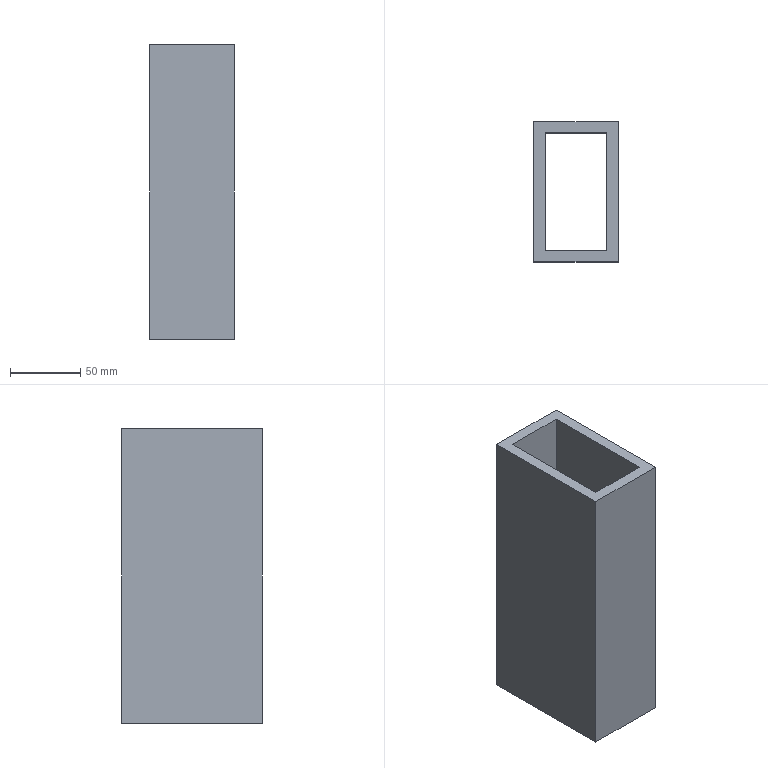Part | SolidWorks | features BaseBody 1 | 1 solid | 10 faces | box 60 x 100 x 210 mm | volume 483840 mm3 | plane 10
STEP:
#1=CARTESIAN_POINT('',(-30.,50.,-105.));
#2=VERTEX_POINT('',#1);
#3=CARTESIAN_POINT('',(-30.,50.,105.));
#4=VERTEX_POINT('',#3);
#5=CARTESIAN_POINT('',(-30.,50.,-105.));
#6=DIRECTION('',(0.,0.,1.));
#7=VECTOR('',#6,1000.);
#8=LINE('',#5,#7);
#9=EDGE_CURVE('',#2,#4,#8,.T.);
#10=ORIENTED_EDGE('',*,*,#9,.F.);
#11=CARTESIAN_POINT('',(-30.,-50.,-105.));
#12=VERTEX_POINT('',#11);
#13=CARTESIAN_POINT('',(-30.,-50.,-105.));
#14=DIRECTION('',(0.,1.,0.));
#15=VECTOR('',#14,1000.);
#16=LINE('',#13,#15);
#17=EDGE_CURVE('',#12,#2,#16,.T.);
#18=ORIENTED_EDGE('',*,*,#17,.F.);
#19=CARTESIAN_POINT('',(-30.,-50.,105.));
#20=VERTEX_POINT('',#19);
#21=CARTESIAN_POINT('',(-30.,-50.,-105.));
#22=DIRECTION('',(0.,0.,-1.));
#23=VECTOR('',#22,1000.);
#24=LINE('',#21,#23);
#25=EDGE_CURVE('',#20,#12,#24,.T.);
#26=ORIENTED_EDGE('',*,*,#25,.F.);
#27=CARTESIAN_POINT('',(-30.,-50.,105.));
#28=DIRECTION('',(0.,-1.,0.));
#29=VECTOR('',#28,1000.);
#30=LINE('',#27,#29);
#31=EDGE_CURVE('',#4,#20,#30,.T.);
#32=ORIENTED_EDGE('',*,*,#31,.F.);
#33=EDGE_LOOP('',(#10,#18,#26,#32));
#34=FACE_OUTER_BOUND('',#33,.T.);
#35=CARTESIAN_POINT('',(-30.,-50.,-105.));
#36=DIRECTION('',(1.,0.,0.));
#37=DIRECTION('',(0.,0.,-1.));
#38=AXIS2_PLACEMENT_3D('',#35,#36,#37);
#39=PLANE('',#38);
#40=ADVANCED_FACE('',(#34),#39,.F.);
#41=CARTESIAN_POINT('',(-22.,42.,105.));
#42=VERTEX_POINT('',#41);
#43=CARTESIAN_POINT('',(22.,42.,105.));
#44=VERTEX_POINT('',#43);
#45=CARTESIAN_POINT('',(-30.,42.,105.));
#46=DIRECTION('',(1.,0.,0.));
#47=VECTOR('',#46,1000.);
#48=LINE('',#45,#47);
#49=EDGE_CURVE('',#42,#44,#48,.T.);
#50=ORIENTED_EDGE('',*,*,#49,.T.);
#51=CARTESIAN_POINT('',(22.,-42.,105.));
#52=VERTEX_POINT('',#51);
#53=CARTESIAN_POINT('',(22.,-50.,105.));
#54=DIRECTION('',(0.,-1.,0.));
#55=VECTOR('',#54,1000.);
#56=LINE('',#53,#55);
#57=EDGE_CURVE('',#44,#52,#56,.T.);
#58=ORIENTED_EDGE('',*,*,#57,.T.);
#59=CARTESIAN_POINT('',(-22.,-42.,105.));
#60=VERTEX_POINT('',#59);
#61=CARTESIAN_POINT('',(-30.,-42.,105.));
#62=DIRECTION('',(-1.,0.,0.));
#63=VECTOR('',#62,1000.);
#64=LINE('',#61,#63);
#65=EDGE_CURVE('',#52,#60,#64,.T.);
#66=ORIENTED_EDGE('',*,*,#65,.T.);
#67=CARTESIAN_POINT('',(-22.,-50.,105.));
#68=DIRECTION('',(0.,1.,0.));
#69=VECTOR('',#68,1000.);
#70=LINE('',#67,#69);
#71=EDGE_CURVE('',#60,#42,#70,.T.);
#72=ORIENTED_EDGE('',*,*,#71,.T.);
#73=EDGE_LOOP('',(#50,#58,#66,#72));
#74=FACE_BOUND('',#73,.T.);
#75=CARTESIAN_POINT('',(30.,-50.,105.));
#76=VERTEX_POINT('',#75);
#77=CARTESIAN_POINT('',(30.,50.,105.));
#78=VERTEX_POINT('',#77);
#79=CARTESIAN_POINT('',(30.,-50.,105.));
#80=DIRECTION('',(0.,1.,0.));
#81=VECTOR('',#80,1000.);
#82=LINE('',#79,#81);
#83=EDGE_CURVE('',#76,#78,#82,.T.);
#84=ORIENTED_EDGE('',*,*,#83,.T.);
#85=CARTESIAN_POINT('',(-30.,50.,105.));
#86=DIRECTION('',(-1.,0.,0.));
#87=VECTOR('',#86,1000.);
#88=LINE('',#85,#87);
#89=EDGE_CURVE('',#78,#4,#88,.T.);
#90=ORIENTED_EDGE('',*,*,#89,.T.);
#91=ORIENTED_EDGE('',*,*,#31,.T.);
#92=CARTESIAN_POINT('',(-30.,-50.,105.));
#93=DIRECTION('',(1.,0.,0.));
#94=VECTOR('',#93,1000.);
#95=LINE('',#92,#94);
#96=EDGE_CURVE('',#20,#76,#95,.T.);
#97=ORIENTED_EDGE('',*,*,#96,.T.);
#98=EDGE_LOOP('',(#84,#90,#91,#97));
#99=FACE_OUTER_BOUND('',#98,.T.);
#100=CARTESIAN_POINT('',(-30.,-50.,105.));
#101=DIRECTION('',(0.,0.,1.));
#102=DIRECTION('',(1.,0.,0.));
#103=AXIS2_PLACEMENT_3D('',#100,#101,#102);
#104=PLANE('',#103);
#105=ADVANCED_FACE('',(#74,#99),#104,.T.);
#106=ORIENTED_EDGE('',*,*,#89,.F.);
#107=CARTESIAN_POINT('',(30.,50.,-105.));
#108=VERTEX_POINT('',#107);
#109=CARTESIAN_POINT('',(30.,50.,-105.));
#110=DIRECTION('',(0.,0.,-1.));
#111=VECTOR('',#110,1000.);
#112=LINE('',#109,#111);
#113=EDGE_CURVE('',#78,#108,#112,.T.);
#114=ORIENTED_EDGE('',*,*,#113,.T.);
#115=CARTESIAN_POINT('',(-30.,50.,-105.));
#116=DIRECTION('',(-1.,0.,0.));
#117=VECTOR('',#116,1000.);
#118=LINE('',#115,#117);
#119=EDGE_CURVE('',#108,#2,#118,.T.);
#120=ORIENTED_EDGE('',*,*,#119,.T.);
#121=ORIENTED_EDGE('',*,*,#9,.T.);
#122=EDGE_LOOP('',(#106,#114,#120,#121));
#123=FACE_OUTER_BOUND('',#122,.T.);
#124=CARTESIAN_POINT('',(-30.,50.,-105.));
#125=DIRECTION('',(0.,1.,0.));
#126=DIRECTION('',(0.,0.,1.));
#127=AXIS2_PLACEMENT_3D('',#124,#125,#126);
#128=PLANE('',#127);
#129=ADVANCED_FACE('',(#123),#128,.T.);
#130=CARTESIAN_POINT('',(-22.,42.,-105.));
#131=VERTEX_POINT('',#130);
#132=CARTESIAN_POINT('',(22.,42.,-105.));
#133=VERTEX_POINT('',#132);
#134=CARTESIAN_POINT('',(-30.,42.,-105.));
#135=DIRECTION('',(1.,0.,0.));
#136=VECTOR('',#135,1000.);
#137=LINE('',#134,#136);
#138=EDGE_CURVE('',#131,#133,#137,.T.);
#139=ORIENTED_EDGE('',*,*,#138,.F.);
#140=CARTESIAN_POINT('',(-22.,-42.,-105.));
#141=VERTEX_POINT('',#140);
#142=CARTESIAN_POINT('',(-22.,-50.,-105.));
#143=DIRECTION('',(0.,1.,0.));
#144=VECTOR('',#143,1000.);
#145=LINE('',#142,#144);
#146=EDGE_CURVE('',#141,#131,#145,.T.);
#147=ORIENTED_EDGE('',*,*,#146,.F.);
#148=CARTESIAN_POINT('',(22.,-42.,-105.));
#149=VERTEX_POINT('',#148);
#150=CARTESIAN_POINT('',(-30.,-42.,-105.));
#151=DIRECTION('',(-1.,0.,0.));
#152=VECTOR('',#151,1000.);
#153=LINE('',#150,#152);
#154=EDGE_CURVE('',#149,#141,#153,.T.);
#155=ORIENTED_EDGE('',*,*,#154,.F.);
#156=CARTESIAN_POINT('',(22.,-50.,-105.));
#157=DIRECTION('',(0.,-1.,0.));
#158=VECTOR('',#157,1000.);
#159=LINE('',#156,#158);
#160=EDGE_CURVE('',#133,#149,#159,.T.);
#161=ORIENTED_EDGE('',*,*,#160,.F.);
#162=EDGE_LOOP('',(#139,#147,#155,#161));
#163=FACE_BOUND('',#162,.T.);
#164=CARTESIAN_POINT('',(30.,-50.,-105.));
#165=VERTEX_POINT('',#164);
#166=CARTESIAN_POINT('',(30.,-50.,-105.));
#167=DIRECTION('',(0.,1.,0.));
#168=VECTOR('',#167,1000.);
#169=LINE('',#166,#168);
#170=EDGE_CURVE('',#165,#108,#169,.T.);
#171=ORIENTED_EDGE('',*,*,#170,.F.);
#172=CARTESIAN_POINT('',(-30.,-50.,-105.));
#173=DIRECTION('',(1.,0.,0.));
#174=VECTOR('',#173,1000.);
#175=LINE('',#172,#174);
#176=EDGE_CURVE('',#12,#165,#175,.T.);
#177=ORIENTED_EDGE('',*,*,#176,.F.);
#178=ORIENTED_EDGE('',*,*,#17,.T.);
#179=ORIENTED_EDGE('',*,*,#119,.F.);
#180=EDGE_LOOP('',(#171,#177,#178,#179));
#181=FACE_OUTER_BOUND('',#180,.T.);
#182=CARTESIAN_POINT('',(-30.,-50.,-105.));
#183=DIRECTION('',(0.,0.,1.));
#184=DIRECTION('',(1.,0.,0.));
#185=AXIS2_PLACEMENT_3D('',#182,#183,#184);
#186=PLANE('',#185);
#187=ADVANCED_FACE('',(#163,#181),#186,.F.);
#188=ORIENTED_EDGE('',*,*,#96,.F.);
#189=ORIENTED_EDGE('',*,*,#25,.T.);
#190=ORIENTED_EDGE('',*,*,#176,.T.);
#191=CARTESIAN_POINT('',(30.,-50.,-105.));
#192=DIRECTION('',(0.,0.,-1.));
#193=VECTOR('',#192,1000.);
#194=LINE('',#191,#193);
#195=EDGE_CURVE('',#76,#165,#194,.T.);
#196=ORIENTED_EDGE('',*,*,#195,.F.);
#197=EDGE_LOOP('',(#188,#189,#190,#196));
#198=FACE_OUTER_BOUND('',#197,.T.);
#199=CARTESIAN_POINT('',(-30.,-50.,-105.));
#200=DIRECTION('',(0.,1.,0.));
#201=DIRECTION('',(0.,0.,1.));
#202=AXIS2_PLACEMENT_3D('',#199,#200,#201);
#203=PLANE('',#202);
#204=ADVANCED_FACE('',(#198),#203,.F.);
#205=CARTESIAN_POINT('',(22.,42.,-106.));
#206=DIRECTION('',(0.,0.,1.));
#207=VECTOR('',#206,1000.);
#208=LINE('',#205,#207);
#209=EDGE_CURVE('',#133,#44,#208,.T.);
#210=ORIENTED_EDGE('',*,*,#209,.F.);
#211=ORIENTED_EDGE('',*,*,#160,.T.);
#212=CARTESIAN_POINT('',(22.,-42.,-106.));
#213=DIRECTION('',(0.,0.,-1.));
#214=VECTOR('',#213,1000.);
#215=LINE('',#212,#214);
#216=EDGE_CURVE('',#52,#149,#215,.T.);
#217=ORIENTED_EDGE('',*,*,#216,.F.);
#218=ORIENTED_EDGE('',*,*,#57,.F.);
#219=EDGE_LOOP('',(#210,#211,#217,#218));
#220=FACE_OUTER_BOUND('',#219,.T.);
#221=CARTESIAN_POINT('',(22.,-42.,-106.));
#222=DIRECTION('',(1.,0.,0.));
#223=DIRECTION('',(0.,0.,-1.));
#224=AXIS2_PLACEMENT_3D('',#221,#222,#223);
#225=PLANE('',#224);
#226=ADVANCED_FACE('',(#220),#225,.F.);
#227=CARTESIAN_POINT('',(-22.,42.,-106.));
#228=DIRECTION('',(0.,0.,1.));
#229=VECTOR('',#228,1000.);
#230=LINE('',#227,#229);
#231=EDGE_CURVE('',#131,#42,#230,.T.);
#232=ORIENTED_EDGE('',*,*,#231,.F.);
#233=ORIENTED_EDGE('',*,*,#138,.T.);
#234=ORIENTED_EDGE('',*,*,#209,.T.);
#235=ORIENTED_EDGE('',*,*,#49,.F.);
#236=EDGE_LOOP('',(#232,#233,#234,#235));
#237=FACE_OUTER_BOUND('',#236,.T.);
#238=CARTESIAN_POINT('',(-22.,42.,-106.));
#239=DIRECTION('',(0.,1.,0.));
#240=DIRECTION('',(0.,0.,1.));
#241=AXIS2_PLACEMENT_3D('',#238,#239,#240);
#242=PLANE('',#241);
#243=ADVANCED_FACE('',(#237),#242,.F.);
#244=ORIENTED_EDGE('',*,*,#231,.T.);
#245=ORIENTED_EDGE('',*,*,#71,.F.);
#246=CARTESIAN_POINT('',(-22.,-42.,-106.));
#247=DIRECTION('',(0.,0.,-1.));
#248=VECTOR('',#247,1000.);
#249=LINE('',#246,#248);
#250=EDGE_CURVE('',#60,#141,#249,.T.);
#251=ORIENTED_EDGE('',*,*,#250,.T.);
#252=ORIENTED_EDGE('',*,*,#146,.T.);
#253=EDGE_LOOP('',(#244,#245,#251,#252));
#254=FACE_OUTER_BOUND('',#253,.T.);
#255=CARTESIAN_POINT('',(-22.,-42.,-106.));
#256=DIRECTION('',(1.,0.,0.));
#257=DIRECTION('',(0.,0.,-1.));
#258=AXIS2_PLACEMENT_3D('',#255,#256,#257);
#259=PLANE('',#258);
#260=ADVANCED_FACE('',(#254),#259,.T.);
#261=ORIENTED_EDGE('',*,*,#250,.F.);
#262=ORIENTED_EDGE('',*,*,#65,.F.);
#263=ORIENTED_EDGE('',*,*,#216,.T.);
#264=ORIENTED_EDGE('',*,*,#154,.T.);
#265=EDGE_LOOP('',(#261,#262,#263,#264));
#266=FACE_OUTER_BOUND('',#265,.T.);
#267=CARTESIAN_POINT('',(-22.,-42.,-106.));
#268=DIRECTION('',(0.,1.,0.));
#269=DIRECTION('',(0.,0.,1.));
#270=AXIS2_PLACEMENT_3D('',#267,#268,#269);
#271=PLANE('',#270);
#272=ADVANCED_FACE('',(#266),#271,.T.);
#273=ORIENTED_EDGE('',*,*,#113,.F.);
#274=ORIENTED_EDGE('',*,*,#83,.F.);
#275=ORIENTED_EDGE('',*,*,#195,.T.);
#276=ORIENTED_EDGE('',*,*,#170,.T.);
#277=EDGE_LOOP('',(#273,#274,#275,#276));
#278=FACE_OUTER_BOUND('',#277,.T.);
#279=CARTESIAN_POINT('',(30.,-50.,-105.));
#280=DIRECTION('',(1.,0.,0.));
#281=DIRECTION('',(0.,0.,-1.));
#282=AXIS2_PLACEMENT_3D('',#279,#280,#281);
#283=PLANE('',#282);
#284=ADVANCED_FACE('',(#278),#283,.T.);
#285=CLOSED_SHELL('',(#40,#105,#129,#187,#204,#226,#243,#260,#272,#284));
#286=MANIFOLD_SOLID_BREP('',#285);
#287=CARTESIAN_POINT('',(0.,0.,0.));
#288=DIRECTION('',(0.,0.,1.));
#289=DIRECTION('',(1.,0.,0.));
#290=AXIS2_PLACEMENT_3D('',#287,#288,#289);
#291=(LENGTH_UNIT()NAMED_UNIT(*)SI_UNIT(.MILLI.,.METRE.));
#292=UNCERTAINTY_MEASURE_WITH_UNIT(LENGTH_MEASURE(0.00001),#291,'','');
#293=(NAMED_UNIT(*)PLANE_ANGLE_UNIT()SI_UNIT($,.RADIAN.));
#294=(NAMED_UNIT(*)SI_UNIT($,.STERADIAN.)SOLID_ANGLE_UNIT());
#295=(GEOMETRIC_REPRESENTATION_CONTEXT(3)GLOBAL_UNCERTAINTY_ASSIGNED_CONTEXT((#292))GLOBAL_UNIT_ASSIGNED_CONTEXT((#291,#293,#294))REPRESENTATION_CONTEXT('',''));
#296=ADVANCED_BREP_SHAPE_REPRESENTATION('',(#286,#290),#295);